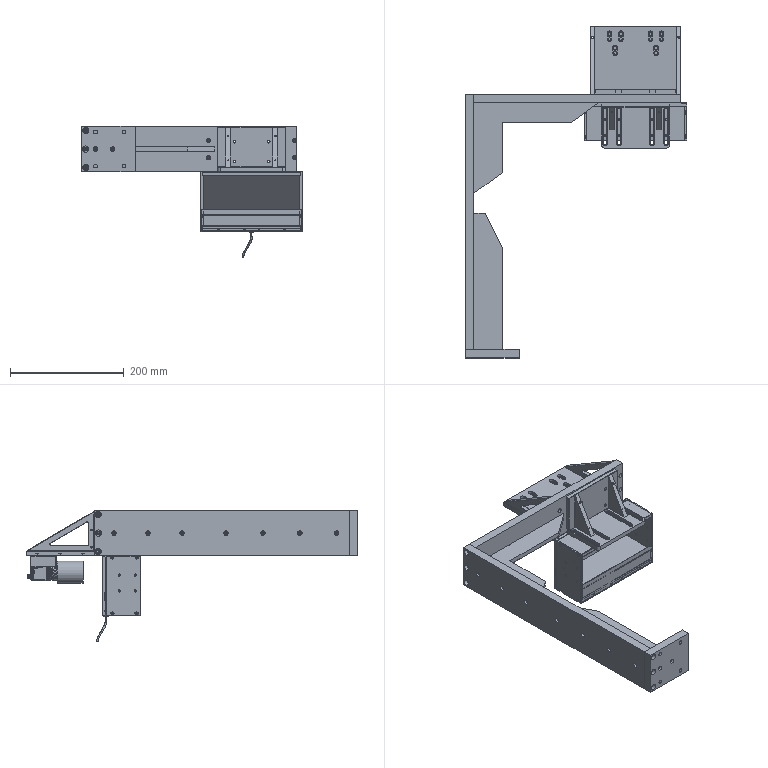Part | SolidWorks | 31 solids | 4496 faces | volume 2167435 mm3 | plane 2316 | cylinder 1364 | cone 462 | spline 348 | torus 6 | commonest cylinder face diameters 0.4 x168 3.3 x100 8 x88 4.5 x80 1.4 x78 2 x60